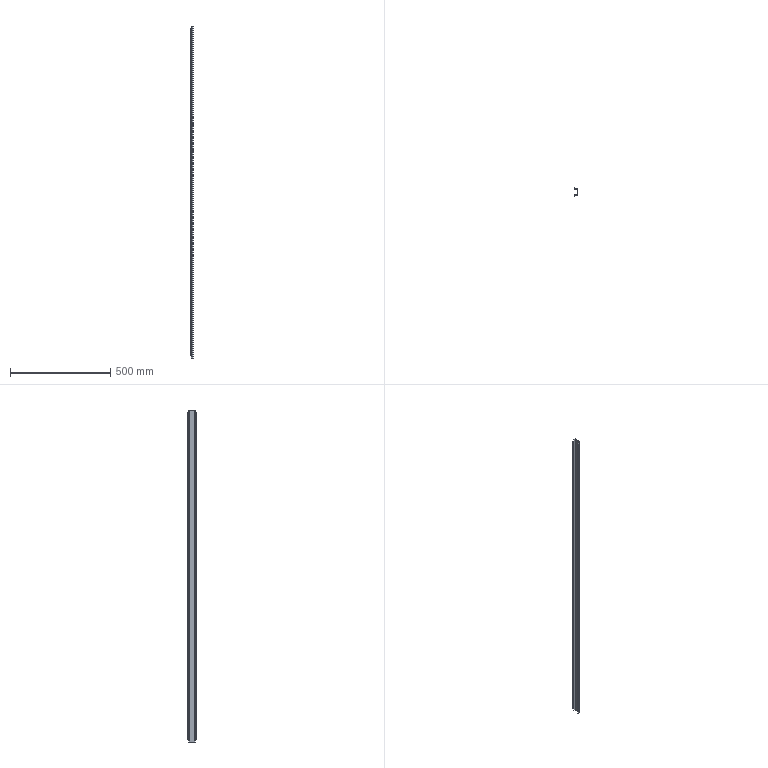Part | STEP file | 1 solid | 102 faces | box 12 x 44 x 1659 mm | volume 107041 mm3 | plane 94 | cylinder 8 | commonest cylinder face diameters 0.4 x4 2.4 x4